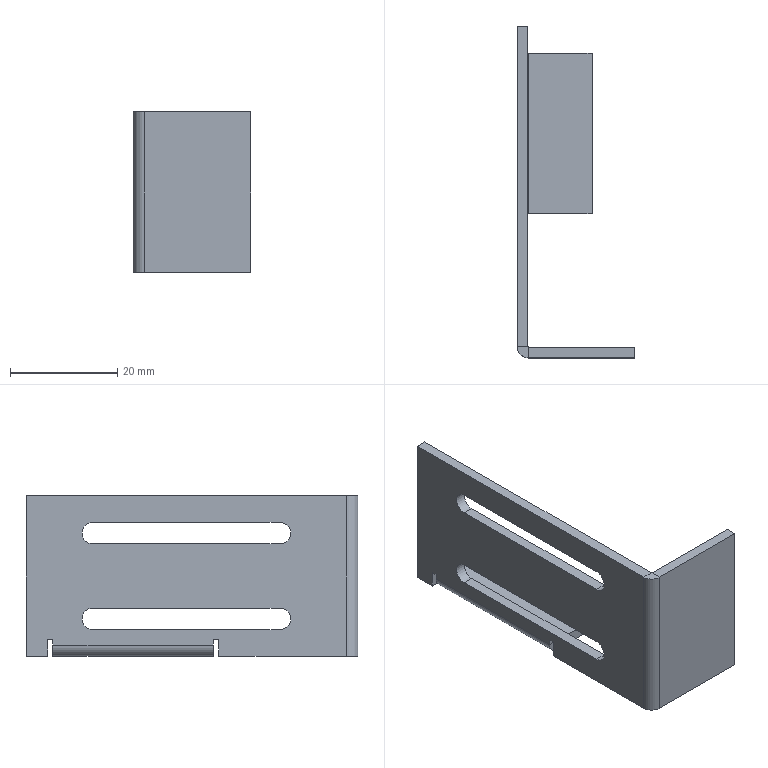Part | SolidWorks | features EdgeFlange 1, FlatPattern 1, ICE 1, SMBaseFlange 1, SheetMetal 1 | 1 solid | 40 faces | box 22 x 62 x 30 mm | volume 4961 mm3 | plane 30 | cylinder 10 | commonest cylinder face diameters 4 x6 0.2 x2 4.2 x2
STEP:
#1=CARTESIAN_POINT('',(0.,12.55,9.));
#2=VERTEX_POINT('',#1);
#3=CARTESIAN_POINT('',(0.,10.55,7.));
#4=VERTEX_POINT('',#3);
#5=CARTESIAN_POINT('',(0.,12.55,7.));
#6=DIRECTION('',(1.,0.,0.));
#7=DIRECTION('',(0.,1.,0.));
#8=AXIS2_PLACEMENT_3D('',#5,#6,#7);
#9=CIRCLE('',#8,2.);
#10=EDGE_CURVE('',#2,#4,#9,.T.);
#11=ORIENTED_EDGE('',*,*,#10,.T.);
#12=CARTESIAN_POINT('',(-2.,10.55,7.));
#13=VERTEX_POINT('',#12);
#14=CARTESIAN_POINT('',(20.,10.55,7.));
#15=DIRECTION('',(-1.,0.,0.));
#16=VECTOR('',#15,1000.);
#17=LINE('',#14,#16);
#18=EDGE_CURVE('',#4,#13,#17,.T.);
#19=ORIENTED_EDGE('',*,*,#18,.T.);
#20=CARTESIAN_POINT('',(-2.,12.55,9.));
#21=VERTEX_POINT('',#20);
#22=CARTESIAN_POINT('',(-2.,12.55,7.));
#23=DIRECTION('',(-1.,0.,0.));
#24=DIRECTION('',(0.,-1.,0.));
#25=AXIS2_PLACEMENT_3D('',#22,#23,#24);
#26=CIRCLE('',#25,2.);
#27=EDGE_CURVE('',#13,#21,#26,.T.);
#28=ORIENTED_EDGE('',*,*,#27,.T.);
#29=CARTESIAN_POINT('',(20.,12.55,9.));
#30=DIRECTION('',(-1.,0.,0.));
#31=VECTOR('',#30,1000.);
#32=LINE('',#29,#31);
#33=EDGE_CURVE('',#2,#21,#32,.T.);
#34=ORIENTED_EDGE('',*,*,#33,.F.);
#35=EDGE_LOOP('',(#11,#19,#28,#34));
#36=FACE_OUTER_BOUND('',#35,.T.);
#37=CARTESIAN_POINT('',(20.,12.55,7.));
#38=DIRECTION('',(-1.,0.,0.));
#39=DIRECTION('',(0.,-1.,0.));
#40=AXIS2_PLACEMENT_3D('',#37,#38,#39);
#41=CYLINDRICAL_SURFACE('',#40,2.);
#42=ADVANCED_FACE('',(#36),#41,.F.);
#43=CARTESIAN_POINT('',(0.,12.55,25.));
#44=VERTEX_POINT('',#43);
#45=CARTESIAN_POINT('',(0.,10.55,23.));
#46=VERTEX_POINT('',#45);
#47=CARTESIAN_POINT('',(0.,12.55,23.));
#48=DIRECTION('',(1.,0.,0.));
#49=DIRECTION('',(0.,1.,0.));
#50=AXIS2_PLACEMENT_3D('',#47,#48,#49);
#51=CIRCLE('',#50,2.);
#52=EDGE_CURVE('',#44,#46,#51,.T.);
#53=ORIENTED_EDGE('',*,*,#52,.T.);
#54=CARTESIAN_POINT('',(-2.,10.55,23.));
#55=VERTEX_POINT('',#54);
#56=CARTESIAN_POINT('',(20.,10.55,23.));
#57=DIRECTION('',(-1.,0.,0.));
#58=VECTOR('',#57,1000.);
#59=LINE('',#56,#58);
#60=EDGE_CURVE('',#46,#55,#59,.T.);
#61=ORIENTED_EDGE('',*,*,#60,.T.);
#62=CARTESIAN_POINT('',(-2.,12.55,25.));
#63=VERTEX_POINT('',#62);
#64=CARTESIAN_POINT('',(-2.,12.55,23.));
#65=DIRECTION('',(-1.,0.,0.));
#66=DIRECTION('',(0.,1.,0.));
#67=AXIS2_PLACEMENT_3D('',#64,#65,#66);
#68=CIRCLE('',#67,2.);
#69=EDGE_CURVE('',#55,#63,#68,.T.);
#70=ORIENTED_EDGE('',*,*,#69,.T.);
#71=CARTESIAN_POINT('',(20.,12.55,25.));
#72=DIRECTION('',(-1.,0.,0.));
#73=VECTOR('',#72,1000.);
#74=LINE('',#71,#73);
#75=EDGE_CURVE('',#44,#63,#74,.T.);
#76=ORIENTED_EDGE('',*,*,#75,.F.);
#77=EDGE_LOOP('',(#53,#61,#70,#76));
#78=FACE_OUTER_BOUND('',#77,.T.);
#79=CARTESIAN_POINT('',(20.,12.55,23.));
#80=DIRECTION('',(-1.,0.,0.));
#81=DIRECTION('',(0.,-1.,0.));
#82=AXIS2_PLACEMENT_3D('',#79,#80,#81);
#83=CYLINDRICAL_SURFACE('',#82,2.);
#84=ADVANCED_FACE('',(#78),#83,.F.);
#85=CARTESIAN_POINT('',(0.,60.,0.));
#86=VERTEX_POINT('',#85);
#87=CARTESIAN_POINT('',(0.,56.,0.));
#88=VERTEX_POINT('',#87);
#89=CARTESIAN_POINT('',(0.,60.,0.));
#90=DIRECTION('',(0.,-1.,0.));
#91=VECTOR('',#90,1000.);
#92=LINE('',#89,#91);
#93=EDGE_CURVE('',#86,#88,#92,.T.);
#94=ORIENTED_EDGE('',*,*,#93,.T.);
#95=CARTESIAN_POINT('',(-2.,56.,0.));
#96=VERTEX_POINT('',#95);
#97=CARTESIAN_POINT('',(0.,56.,0.));
#98=DIRECTION('',(-1.,0.,0.));
#99=VECTOR('',#98,1000.);
#100=LINE('',#97,#99);
#101=EDGE_CURVE('',#88,#96,#100,.T.);
#102=ORIENTED_EDGE('',*,*,#101,.T.);
#103=CARTESIAN_POINT('',(-2.,60.,0.));
#104=VERTEX_POINT('',#103);
#105=CARTESIAN_POINT('',(-2.,60.,0.));
#106=DIRECTION('',(0.,-1.,0.));
#107=VECTOR('',#106,1000.);
#108=LINE('',#105,#107);
#109=EDGE_CURVE('',#104,#96,#108,.T.);
#110=ORIENTED_EDGE('',*,*,#109,.F.);
#111=CARTESIAN_POINT('',(-2.,60.,0.));
#112=DIRECTION('',(1.,0.,0.));
#113=VECTOR('',#112,1000.);
#114=LINE('',#111,#113);
#115=EDGE_CURVE('',#104,#86,#114,.T.);
#116=ORIENTED_EDGE('',*,*,#115,.T.);
#117=EDGE_LOOP('',(#94,#102,#110,#116));
#118=FACE_OUTER_BOUND('',#117,.T.);
#119=CARTESIAN_POINT('',(0.1,-2.,0.));
#120=DIRECTION('',(0.,0.,-1.));
#121=DIRECTION('',(-1.,0.,0.));
#122=AXIS2_PLACEMENT_3D('',#119,#120,#121);
#123=PLANE('',#122);
#124=ADVANCED_FACE('',(#118),#123,.T.);
#125=CARTESIAN_POINT('',(-2.,24.,0.));
#126=VERTEX_POINT('',#125);
#127=CARTESIAN_POINT('',(-2.,0.1,0.));
#128=VERTEX_POINT('',#127);
#129=CARTESIAN_POINT('',(-2.,60.,0.));
#130=DIRECTION('',(0.,-1.,0.));
#131=VECTOR('',#130,1000.);
#132=LINE('',#129,#131);
#133=EDGE_CURVE('',#126,#128,#132,.T.);
#134=ORIENTED_EDGE('',*,*,#133,.F.);
#135=CARTESIAN_POINT('',(0.,24.,0.));
#136=VERTEX_POINT('',#135);
#137=CARTESIAN_POINT('',(0.,24.,0.));
#138=DIRECTION('',(-1.,0.,0.));
#139=VECTOR('',#138,1000.);
#140=LINE('',#137,#139);
#141=EDGE_CURVE('',#136,#126,#140,.T.);
#142=ORIENTED_EDGE('',*,*,#141,.F.);
#143=CARTESIAN_POINT('',(0.,0.1,0.));
#144=VERTEX_POINT('',#143);
#145=CARTESIAN_POINT('',(0.,60.,0.));
#146=DIRECTION('',(0.,-1.,0.));
#147=VECTOR('',#146,1000.);
#148=LINE('',#145,#147);
#149=EDGE_CURVE('',#136,#144,#148,.T.);
#150=ORIENTED_EDGE('',*,*,#149,.T.);
#151=CARTESIAN_POINT('',(0.,0.1,0.));
#152=DIRECTION('',(-1.,0.,0.));
#153=VECTOR('',#152,1000.);
#154=LINE('',#151,#153);
#155=EDGE_CURVE('',#144,#128,#154,.T.);
#156=ORIENTED_EDGE('',*,*,#155,.T.);
#157=EDGE_LOOP('',(#134,#142,#150,#156));
#158=FACE_OUTER_BOUND('',#157,.T.);
#159=CARTESIAN_POINT('',(0.1,-2.,0.));
#160=DIRECTION('',(0.,0.,-1.));
#161=DIRECTION('',(-1.,0.,0.));
#162=AXIS2_PLACEMENT_3D('',#159,#160,#161);
#163=PLANE('',#162);
#164=ADVANCED_FACE('',(#158),#163,.T.);
#165=CARTESIAN_POINT('',(0.,47.55,5.));
#166=VERTEX_POINT('',#165);
#167=CARTESIAN_POINT('',(0.,47.55,9.));
#168=VERTEX_POINT('',#167);
#169=CARTESIAN_POINT('',(0.,47.55,7.));
#170=DIRECTION('',(1.,0.,0.));
#171=DIRECTION('',(0.,1.,0.));
#172=AXIS2_PLACEMENT_3D('',#169,#170,#171);
#173=CIRCLE('',#172,2.);
#174=EDGE_CURVE('',#166,#168,#173,.T.);
#175=ORIENTED_EDGE('',*,*,#174,.F.);
#176=CARTESIAN_POINT('',(0.,12.55,5.));
#177=VERTEX_POINT('',#176);
#178=CARTESIAN_POINT('',(0.,60.,5.));
#179=DIRECTION('',(0.,1.,0.));
#180=VECTOR('',#179,1000.);
#181=LINE('',#178,#180);
#182=EDGE_CURVE('',#177,#166,#181,.T.);
#183=ORIENTED_EDGE('',*,*,#182,.F.);
#184=CARTESIAN_POINT('',(0.,12.55,7.));
#185=DIRECTION('',(1.,0.,0.));
#186=DIRECTION('',(0.,1.,0.));
#187=AXIS2_PLACEMENT_3D('',#184,#185,#186);
#188=CIRCLE('',#187,2.);
#189=EDGE_CURVE('',#4,#177,#188,.T.);
#190=ORIENTED_EDGE('',*,*,#189,.F.);
#191=ORIENTED_EDGE('',*,*,#10,.F.);
#192=CARTESIAN_POINT('',(0.,60.,9.));
#193=DIRECTION('',(0.,-1.,0.));
#194=VECTOR('',#193,1000.);
#195=LINE('',#192,#194);
#196=EDGE_CURVE('',#168,#2,#195,.T.);
#197=ORIENTED_EDGE('',*,*,#196,.F.);
#198=EDGE_LOOP('',(#175,#183,#190,#191,#197));
#199=FACE_BOUND('',#198,.T.);
#200=CARTESIAN_POINT('',(0.,47.55,21.));
#201=VERTEX_POINT('',#200);
#202=CARTESIAN_POINT('',(0.,47.55,25.));
#203=VERTEX_POINT('',#202);
#204=CARTESIAN_POINT('',(0.,47.55,23.));
#205=DIRECTION('',(1.,0.,0.));
#206=DIRECTION('',(0.,1.,0.));
#207=AXIS2_PLACEMENT_3D('',#204,#205,#206);
#208=CIRCLE('',#207,2.);
#209=EDGE_CURVE('',#201,#203,#208,.T.);
#210=ORIENTED_EDGE('',*,*,#209,.F.);
#211=CARTESIAN_POINT('',(0.,12.55,21.));
#212=VERTEX_POINT('',#211);
#213=CARTESIAN_POINT('',(0.,60.,21.));
#214=DIRECTION('',(0.,1.,0.));
#215=VECTOR('',#214,1000.);
#216=LINE('',#213,#215);
#217=EDGE_CURVE('',#212,#201,#216,.T.);
#218=ORIENTED_EDGE('',*,*,#217,.F.);
#219=CARTESIAN_POINT('',(0.,12.55,23.));
#220=DIRECTION('',(1.,0.,0.));
#221=DIRECTION('',(0.,1.,0.));
#222=AXIS2_PLACEMENT_3D('',#219,#220,#221);
#223=CIRCLE('',#222,2.);
#224=EDGE_CURVE('',#46,#212,#223,.T.);
#225=ORIENTED_EDGE('',*,*,#224,.F.);
#226=ORIENTED_EDGE('',*,*,#52,.F.);
#227=CARTESIAN_POINT('',(0.,60.,25.));
#228=DIRECTION('',(0.,-1.,0.));
#229=VECTOR('',#228,1000.);
#230=LINE('',#227,#229);
#231=EDGE_CURVE('',#203,#44,#230,.T.);
#232=ORIENTED_EDGE('',*,*,#231,.F.);
#233=EDGE_LOOP('',(#210,#218,#225,#226,#232));
#234=FACE_BOUND('',#233,.T.);
#235=CARTESIAN_POINT('',(0.,56.,3.1));
#236=VERTEX_POINT('',#235);
#237=CARTESIAN_POINT('',(0.,55.,3.1));
#238=VERTEX_POINT('',#237);
#239=CARTESIAN_POINT('',(0.,56.,3.1));
#240=DIRECTION('',(0.,-1.,0.));
#241=VECTOR('',#240,1000.);
#242=LINE('',#239,#241);
#243=EDGE_CURVE('',#236,#238,#242,.T.);
#244=ORIENTED_EDGE('',*,*,#243,.F.);
#245=CARTESIAN_POINT('',(0.,56.,0.));
#246=DIRECTION('',(0.,0.,1.));
#247=VECTOR('',#246,1000.);
#248=LINE('',#245,#247);
#249=EDGE_CURVE('',#88,#236,#248,.T.);
#250=ORIENTED_EDGE('',*,*,#249,.F.);
#251=ORIENTED_EDGE('',*,*,#93,.F.);
#252=CARTESIAN_POINT('',(0.,60.,30.));
#253=VERTEX_POINT('',#252);
#254=CARTESIAN_POINT('',(0.,60.,30.));
#255=DIRECTION('',(0.,0.,-1.));
#256=VECTOR('',#255,1000.);
#257=LINE('',#254,#256);
#258=EDGE_CURVE('',#253,#86,#257,.T.);
#259=ORIENTED_EDGE('',*,*,#258,.F.);
#260=CARTESIAN_POINT('',(0.,0.1,30.));
#261=VERTEX_POINT('',#260);
#262=CARTESIAN_POINT('',(0.,60.,30.));
#263=DIRECTION('',(0.,-1.,0.));
#264=VECTOR('',#263,1000.);
#265=LINE('',#262,#264);
#266=EDGE_CURVE('',#253,#261,#265,.T.);
#267=ORIENTED_EDGE('',*,*,#266,.T.);
#268=CARTESIAN_POINT('',(0.,0.1,30.));
#269=DIRECTION('',(0.,0.,-1.));
#270=VECTOR('',#269,1000.);
#271=LINE('',#268,#270);
#272=EDGE_CURVE('',#261,#144,#271,.T.);
#273=ORIENTED_EDGE('',*,*,#272,.T.);
#274=ORIENTED_EDGE('',*,*,#149,.F.);
#275=CARTESIAN_POINT('',(0.,24.,3.1));
#276=VERTEX_POINT('',#275);
#277=CARTESIAN_POINT('',(0.,24.,3.1));
#278=DIRECTION('',(0.,0.,-1.));
#279=VECTOR('',#278,1000.);
#280=LINE('',#277,#279);
#281=EDGE_CURVE('',#276,#136,#280,.T.);
#282=ORIENTED_EDGE('',*,*,#281,.F.);
#283=CARTESIAN_POINT('',(0.,25.,3.1));
#284=VERTEX_POINT('',#283);
#285=CARTESIAN_POINT('',(0.,25.,3.1));
#286=DIRECTION('',(0.,-1.,0.));
#287=VECTOR('',#286,1000.);
#288=LINE('',#285,#287);
#289=EDGE_CURVE('',#284,#276,#288,.T.);
#290=ORIENTED_EDGE('',*,*,#289,.F.);
#291=CARTESIAN_POINT('',(0.,25.,2.1));
#292=VERTEX_POINT('',#291);
#293=CARTESIAN_POINT('',(0.,25.,2.1));
#294=DIRECTION('',(0.,0.,1.));
#295=VECTOR('',#294,1000.);
#296=LINE('',#293,#295);
#297=EDGE_CURVE('',#292,#284,#296,.T.);
#298=ORIENTED_EDGE('',*,*,#297,.F.);
#299=CARTESIAN_POINT('',(0.,55.,2.1));
#300=VERTEX_POINT('',#299);
#301=CARTESIAN_POINT('',(0.,55.,2.1));
#302=DIRECTION('',(0.,-1.,0.));
#303=VECTOR('',#302,1000.);
#304=LINE('',#301,#303);
#305=EDGE_CURVE('',#300,#292,#304,.T.);
#306=ORIENTED_EDGE('',*,*,#305,.F.);
#307=CARTESIAN_POINT('',(0.,55.,3.1));
#308=DIRECTION('',(0.,0.,-1.));
#309=VECTOR('',#308,1000.);
#310=LINE('',#307,#309);
#311=EDGE_CURVE('',#238,#300,#310,.T.);
#312=ORIENTED_EDGE('',*,*,#311,.F.);
#313=EDGE_LOOP('',(#244,#250,#251,#259,#267,#273,#274,#282,#290,#298,#306,#312));
#314=FACE_OUTER_BOUND('',#313,.T.);
#315=CARTESIAN_POINT('',(0.,60.,30.));
#316=DIRECTION('',(1.,0.,0.));
#317=DIRECTION('',(0.,1.,0.));
#318=AXIS2_PLACEMENT_3D('',#315,#316,#317);
#319=PLANE('',#318);
#320=ADVANCED_FACE('',(#199,#234,#314),#319,.T.);
#321=CARTESIAN_POINT('',(-2.,47.55,21.));
#322=VERTEX_POINT('',#321);
#323=CARTESIAN_POINT('',(-2.,12.55,21.));
#324=VERTEX_POINT('',#323);
#325=CARTESIAN_POINT('',(-2.,47.55,21.));
#326=DIRECTION('',(0.,-1.,0.));
#327=VECTOR('',#326,1000.);
#328=LINE('',#325,#327);
#329=EDGE_CURVE('',#322,#324,#328,.T.);
#330=ORIENTED_EDGE('',*,*,#329,.F.);
#331=CARTESIAN_POINT('',(-2.,47.55,25.));
#332=VERTEX_POINT('',#331);
#333=CARTESIAN_POINT('',(-2.,47.55,23.));
#334=DIRECTION('',(-1.,0.,0.));
#335=DIRECTION('',(0.,1.,0.));
#336=AXIS2_PLACEMENT_3D('',#333,#334,#335);
#337=CIRCLE('',#336,2.);
#338=EDGE_CURVE('',#332,#322,#337,.T.);
#339=ORIENTED_EDGE('',*,*,#338,.F.);
#340=CARTESIAN_POINT('',(-2.,47.55,25.));
#341=DIRECTION('',(0.,1.,0.));
#342=VECTOR('',#341,1000.);
#343=LINE('',#340,#342);
#344=EDGE_CURVE('',#63,#332,#343,.T.);
#345=ORIENTED_EDGE('',*,*,#344,.F.);
#346=ORIENTED_EDGE('',*,*,#69,.F.);
#347=CARTESIAN_POINT('',(-2.,12.55,23.));
#348=DIRECTION('',(-1.,0.,0.));
#349=DIRECTION('',(0.,1.,0.));
#350=AXIS2_PLACEMENT_3D('',#347,#348,#349);
#351=CIRCLE('',#350,2.);
#352=EDGE_CURVE('',#324,#55,#351,.T.);
#353=ORIENTED_EDGE('',*,*,#352,.F.);
#354=EDGE_LOOP('',(#330,#339,#345,#346,#353));
#355=FACE_BOUND('',#354,.T.);
#356=CARTESIAN_POINT('',(-2.,47.55,5.));
#357=VERTEX_POINT('',#356);
#358=CARTESIAN_POINT('',(-2.,12.55,5.));
#359=VERTEX_POINT('',#358);
#360=CARTESIAN_POINT('',(-2.,47.55,5.));
#361=DIRECTION('',(0.,-1.,0.));
#362=VECTOR('',#361,1000.);
#363=LINE('',#360,#362);
#364=EDGE_CURVE('',#357,#359,#363,.T.);
#365=ORIENTED_EDGE('',*,*,#364,.F.);
#366=CARTESIAN_POINT('',(-2.,47.55,9.));
#367=VERTEX_POINT('',#366);
#368=CARTESIAN_POINT('',(-2.,47.55,7.));
#369=DIRECTION('',(-1.,0.,0.));
#370=DIRECTION('',(0.,-1.,0.));
#371=AXIS2_PLACEMENT_3D('',#368,#369,#370);
#372=CIRCLE('',#371,2.);
#373=EDGE_CURVE('',#367,#357,#372,.T.);
#374=ORIENTED_EDGE('',*,*,#373,.F.);
#375=CARTESIAN_POINT('',(-2.,47.55,9.));
#376=DIRECTION('',(0.,1.,0.));
#377=VECTOR('',#376,1000.);
#378=LINE('',#375,#377);
#379=EDGE_CURVE('',#21,#367,#378,.T.);
#380=ORIENTED_EDGE('',*,*,#379,.F.);
#381=ORIENTED_EDGE('',*,*,#27,.F.);
#382=CARTESIAN_POINT('',(-2.,12.55,7.));
#383=DIRECTION('',(-1.,0.,0.));
#384=DIRECTION('',(0.,-1.,0.));
#385=AXIS2_PLACEMENT_3D('',#382,#383,#384);
#386=CIRCLE('',#385,2.);
#387=EDGE_CURVE('',#359,#13,#386,.T.);
#388=ORIENTED_EDGE('',*,*,#387,.F.);
#389=EDGE_LOOP('',(#365,#374,#380,#381,#388));
#390=FACE_BOUND('',#389,.T.);
#391=CARTESIAN_POINT('',(-2.,56.,3.1));
#392=VERTEX_POINT('',#391);
#393=CARTESIAN_POINT('',(-2.,56.,30.));
#394=DIRECTION('',(0.,0.,-1.));
#395=VECTOR('',#394,1000.);
#396=LINE('',#393,#395);
#397=EDGE_CURVE('',#392,#96,#396,.T.);
#398=ORIENTED_EDGE('',*,*,#397,.F.);
#399=CARTESIAN_POINT('',(-2.,55.,3.1));
#400=VERTEX_POINT('',#399);
#401=CARTESIAN_POINT('',(-2.,60.,3.1));
#402=DIRECTION('',(0.,1.,0.));
#403=VECTOR('',#402,1000.);
#404=LINE('',#401,#403);
#405=EDGE_CURVE('',#400,#392,#404,.T.);
#406=ORIENTED_EDGE('',*,*,#405,.F.);
#407=CARTESIAN_POINT('',(-2.,55.,2.1));
#408=VERTEX_POINT('',#407);
#409=CARTESIAN_POINT('',(-2.,55.,30.));
#410=DIRECTION('',(0.,0.,1.));
#411=VECTOR('',#410,1000.);
#412=LINE('',#409,#411);
#413=EDGE_CURVE('',#408,#400,#412,.T.);
#414=ORIENTED_EDGE('',*,*,#413,.F.);
#415=CARTESIAN_POINT('',(-2.,25.,2.1));
#416=VERTEX_POINT('',#415);
#417=CARTESIAN_POINT('',(-2.,55.,2.1));
#418=DIRECTION('',(0.,-1.,0.));
#419=VECTOR('',#418,1000.);
#420=LINE('',#417,#419);
#421=EDGE_CURVE('',#408,#416,#420,.T.);
#422=ORIENTED_EDGE('',*,*,#421,.T.);
#423=CARTESIAN_POINT('',(-2.,25.,3.1));
#424=VERTEX_POINT('',#423);
#425=CARTESIAN_POINT('',(-2.,25.,30.));
#426=DIRECTION('',(0.,0.,-1.));
#427=VECTOR('',#426,1000.);
#428=LINE('',#425,#427);
#429=EDGE_CURVE('',#424,#416,#428,.T.);
#430=ORIENTED_EDGE('',*,*,#429,.F.);
#431=CARTESIAN_POINT('',(-2.,24.,3.1));
#432=VERTEX_POINT('',#431);
#433=CARTESIAN_POINT('',(-2.,60.,3.1));
#434=DIRECTION('',(0.,1.,0.));
#435=VECTOR('',#434,1000.);
#436=LINE('',#433,#435);
#437=EDGE_CURVE('',#432,#424,#436,.T.);
#438=ORIENTED_EDGE('',*,*,#437,.F.);
#439=CARTESIAN_POINT('',(-2.,24.,30.));
#440=DIRECTION('',(0.,0.,1.));
#441=VECTOR('',#440,1000.);
#442=LINE('',#439,#441);
#443=EDGE_CURVE('',#126,#432,#442,.T.);
#444=ORIENTED_EDGE('',*,*,#443,.F.);
#445=ORIENTED_EDGE('',*,*,#133,.T.);
#446=CARTESIAN_POINT('',(-2.,0.1,30.));
#447=VERTEX_POINT('',#446);
#448=CARTESIAN_POINT('',(-2.,0.1,30.));
#449=DIRECTION('',(0.,0.,-1.));
#450=VECTOR('',#449,1000.);
#451=LINE('',#448,#450);
#452=EDGE_CURVE('',#447,#128,#451,.T.);
#453=ORIENTED_EDGE('',*,*,#452,.F.);
#454=CARTESIAN_POINT('',(-2.,60.,30.));
#455=VERTEX_POINT('',#454);
#456=CARTESIAN_POINT('',(-2.,60.,30.));
#457=DIRECTION('',(0.,-1.,0.));
#458=VECTOR('',#457,1000.);
#459=LINE('',#456,#458);
#460=EDGE_CURVE('',#455,#447,#459,.T.);
#461=ORIENTED_EDGE('',*,*,#460,.F.);
#462=CARTESIAN_POINT('',(-2.,60.,30.));
#463=DIRECTION('',(0.,0.,-1.));
#464=VECTOR('',#463,1000.);
#465=LINE('',#462,#464);
#466=EDGE_CURVE('',#455,#104,#465,.T.);
#467=ORIENTED_EDGE('',*,*,#466,.T.);
#468=ORIENTED_EDGE('',*,*,#109,.T.);
#469=EDGE_LOOP('',(#398,#406,#414,#422,#430,#438,#444,#445,#453,#461,#467,#468));
#470=FACE_OUTER_BOUND('',#469,.T.);
#471=CARTESIAN_POINT('',(-2.,60.,30.));
#472=DIRECTION('',(1.,0.,0.));
#473=DIRECTION('',(0.,1.,0.));
#474=AXIS2_PLACEMENT_3D('',#471,#472,#473);
#475=PLANE('',#474);
#476=ADVANCED_FACE('',(#355,#390,#470),#475,.F.);
#477=CARTESIAN_POINT('',(0.1,0.,30.));
#478=VERTEX_POINT('',#477);
#479=CARTESIAN_POINT('',(0.1,-2.,30.));
#480=VERTEX_POINT('',#479);
#481=CARTESIAN_POINT('',(0.1,0.,30.));
#482=DIRECTION('',(0.,-1.,0.));
#483=VECTOR('',#482,1000.);
#484=LINE('',#481,#483);
#485=EDGE_CURVE('',#478,#480,#484,.T.);
#486=ORIENTED_EDGE('',*,*,#485,.F.);
#487=CARTESIAN_POINT('',(0.1,0.1,30.));
#488=DIRECTION('',(0.,0.,1.));
#489=DIRECTION('',(-1.,0.,0.));
#490=AXIS2_PLACEMENT_3D('',#487,#488,#489);
#491=CIRCLE('',#490,0.1);
#492=EDGE_CURVE('',#261,#478,#491,.T.);
#493=ORIENTED_EDGE('',*,*,#492,.F.);
#494=CARTESIAN_POINT('',(-2.,0.1,30.));
#495=DIRECTION('',(1.,0.,0.));
#496=VECTOR('',#495,1000.);
#497=LINE('',#494,#496);
#498=EDGE_CURVE('',#447,#261,#497,.T.);
#499=ORIENTED_EDGE('',*,*,#498,.F.);
#500=CARTESIAN_POINT('',(0.1,0.1,30.));
#501=DIRECTION('',(0.,0.,1.));
#502=DIRECTION('',(1.,0.,0.));
#503=AXIS2_PLACEMENT_3D('',#500,#501,#502);
#504=CIRCLE('',#503,2.1);
#505=EDGE_CURVE('',#447,#480,#504,.T.);
#506=ORIENTED_EDGE('',*,*,#505,.T.);
#507=EDGE_LOOP('',(#486,#493,#499,#506));
#508=FACE_OUTER_BOUND('',#507,.T.);
#509=CARTESIAN_POINT('',(0.1,0.,30.));
#510=DIRECTION('',(0.,0.,1.));
#511=DIRECTION('',(1.,0.,0.));
#512=AXIS2_PLACEMENT_3D('',#509,#510,#511);
#513=PLANE('',#512);
#514=ADVANCED_FACE('',(#508),#513,.T.);
#515=CARTESIAN_POINT('',(20.,0.,30.));
#516=VERTEX_POINT('',#515);
#517=CARTESIAN_POINT('',(0.,0.,30.));
#518=DIRECTION('',(1.,0.,0.));
#519=VECTOR('',#518,1000.);
#520=LINE('',#517,#519);
#521=EDGE_CURVE('',#478,#516,#520,.T.);
#522=ORIENTED_EDGE('',*,*,#521,.F.);
#523=ORIENTED_EDGE('',*,*,#485,.T.);
#524=CARTESIAN_POINT('',(20.,-2.,30.));
#525=VERTEX_POINT('',#524);
#526=CARTESIAN_POINT('',(0.,-2.,30.));
#527=DIRECTION('',(1.,0.,0.));
#528=VECTOR('',#527,1000.);
#529=LINE('',#526,#528);
#530=EDGE_CURVE('',#480,#525,#529,.T.);
#531=ORIENTED_EDGE('',*,*,#530,.T.);
#532=CARTESIAN_POINT('',(20.,0.,30.));
#533=DIRECTION('',(0.,-1.,0.));
#534=VECTOR('',#533,1000.);
#535=LINE('',#532,#534);
#536=EDGE_CURVE('',#516,#525,#535,.T.);
#537=ORIENTED_EDGE('',*,*,#536,.F.);
#538=EDGE_LOOP('',(#522,#523,#531,#537));
#539=FACE_OUTER_BOUND('',#538,.T.);
#540=CARTESIAN_POINT('',(-2.,0.1,30.));
#541=DIRECTION('',(0.,0.,1.));
#542=DIRECTION('',(1.,0.,0.));
#543=AXIS2_PLACEMENT_3D('',#540,#541,#542);
#544=PLANE('',#543);
#545=ADVANCED_FACE('',(#539),#544,.T.);
#546=ORIENTED_EDGE('',*,*,#155,.F.);
#547=CARTESIAN_POINT('',(0.1,0.,0.));
#548=VERTEX_POINT('',#547);
#549=CARTESIAN_POINT('',(0.1,0.1,0.));
#550=DIRECTION('',(0.,0.,1.));
#551=DIRECTION('',(-1.,0.,0.));
#552=AXIS2_PLACEMENT_3D('',#549,#550,#551);
#553=CIRCLE('',#552,0.1);
#554=EDGE_CURVE('',#144,#548,#553,.T.);
#555=ORIENTED_EDGE('',*,*,#554,.T.);
#556=CARTESIAN_POINT('',(0.1,-2.,0.));
#557=VERTEX_POINT('',#556);
#558=CARTESIAN_POINT('',(0.1,-2.,0.));
#559=DIRECTION('',(0.,1.,0.));
#560=VECTOR('',#559,1000.);
#561=LINE('',#558,#560);
#562=EDGE_CURVE('',#557,#548,#561,.T.);
#563=ORIENTED_EDGE('',*,*,#562,.F.);
#564=CARTESIAN_POINT('',(0.1,0.1,0.));
#565=DIRECTION('',(0.,0.,1.));
#566=DIRECTION('',(1.,0.,0.));
#567=AXIS2_PLACEMENT_3D('',#564,#565,#566);
#568=CIRCLE('',#567,2.1);
#569=EDGE_CURVE('',#128,#557,#568,.T.);
#570=ORIENTED_EDGE('',*,*,#569,.F.);
#571=EDGE_LOOP('',(#546,#555,#563,#570));
#572=FACE_OUTER_BOUND('',#571,.T.);
#573=CARTESIAN_POINT('',(0.,0.1,0.));
#574=DIRECTION('',(0.,0.,-1.));
#575=DIRECTION('',(-1.,0.,0.));
#576=AXIS2_PLACEMENT_3D('',#573,#574,#575);
#577=PLANE('',#576);
#578=ADVANCED_FACE('',(#572),#577,.T.);
#579=CARTESIAN_POINT('',(20.,-2.,0.));
#580=VERTEX_POINT('',#579);
#581=CARTESIAN_POINT('',(0.,-2.,0.));
#582=DIRECTION('',(1.,0.,0.));
#583=VECTOR('',#582,1000.);
#584=LINE('',#581,#583);
#585=EDGE_CURVE('',#557,#580,#584,.T.);
#586=ORIENTED_EDGE('',*,*,#585,.T.);
#587=CARTESIAN_POINT('',(20.,-2.,30.));
#588=DIRECTION('',(0.,0.,-1.));
#589=VECTOR('',#588,1000.);
#590=LINE('',#587,#589);
#591=EDGE_CURVE('',#525,#580,#590,.T.);
#592=ORIENTED_EDGE('',*,*,#591,.F.);
#593=ORIENTED_EDGE('',*,*,#530,.F.);
#594=CARTESIAN_POINT('',(0.1,-2.,30.));
#595=DIRECTION('',(0.,0.,-1.));
#596=VECTOR('',#595,1000.);
#597=LINE('',#594,#596);
#598=EDGE_CURVE('',#480,#557,#597,.T.);
#599=ORIENTED_EDGE('',*,*,#598,.T.);
#600=EDGE_LOOP('',(#586,#592,#593,#599));
#601=FACE_OUTER_BOUND('',#600,.T.);
#602=CARTESIAN_POINT('',(0.,-2.,30.));
#603=DIRECTION('',(0.,1.,0.));
#604=DIRECTION('',(0.,0.,1.));
#605=AXIS2_PLACEMENT_3D('',#602,#603,#604);
#606=PLANE('',#605);
#607=ADVANCED_FACE('',(#601),#606,.F.);
#608=CARTESIAN_POINT('',(20.,0.,0.));
#609=VERTEX_POINT('',#608);
#610=CARTESIAN_POINT('',(20.,0.,0.));
#611=DIRECTION('',(0.,-1.,0.));
#612=VECTOR('',#611,1000.);
#613=LINE('',#610,#612);
#614=EDGE_CURVE('',#609,#580,#613,.T.);
#615=ORIENTED_EDGE('',*,*,#614,.F.);
#616=CARTESIAN_POINT('',(20.,0.,30.));
#617=DIRECTION('',(0.,0.,-1.));
#618=VECTOR('',#617,1000.);
#619=LINE('',#616,#618);
#620=EDGE_CURVE('',#516,#609,#619,.T.);
#621=ORIENTED_EDGE('',*,*,#620,.F.);
#622=ORIENTED_EDGE('',*,*,#536,.T.);
#623=ORIENTED_EDGE('',*,*,#591,.T.);
#624=EDGE_LOOP('',(#615,#621,#622,#623));
#625=FACE_OUTER_BOUND('',#624,.T.);
#626=CARTESIAN_POINT('',(20.,0.,30.));
#627=DIRECTION('',(1.,0.,0.));
#628=DIRECTION('',(0.,0.,-1.));
#629=AXIS2_PLACEMENT_3D('',#626,#627,#628);
#630=PLANE('',#629);
#631=ADVANCED_FACE('',(#625),#630,.T.);
#632=CARTESIAN_POINT('',(0.,0.,0.));
#633=DIRECTION('',(1.,0.,0.));
#634=VECTOR('',#633,1000.);
#635=LINE('',#632,#634);
#636=EDGE_CURVE('',#548,#609,#635,.T.);
#637=ORIENTED_EDGE('',*,*,#636,.F.);
#638=CARTESIAN_POINT('',(0.1,0.,30.));
#639=DIRECTION('',(0.,0.,-1.));
#640=VECTOR('',#639,1000.);
#641=LINE('',#638,#640);
#642=EDGE_CURVE('',#478,#548,#641,.T.);
#643=ORIENTED_EDGE('',*,*,#642,.F.);
#644=ORIENTED_EDGE('',*,*,#521,.T.);
#645=ORIENTED_EDGE('',*,*,#620,.T.);
#646=EDGE_LOOP('',(#637,#643,#644,#645));
#647=FACE_OUTER_BOUND('',#646,.T.);
#648=CARTESIAN_POINT('',(0.,0.,30.));
#649=DIRECTION('',(0.,1.,0.));
#650=DIRECTION('',(0.,0.,1.));
#651=AXIS2_PLACEMENT_3D('',#648,#649,#650);
#652=PLANE('',#651);
#653=ADVANCED_FACE('',(#647),#652,.T.);
#654=ORIENTED_EDGE('',*,*,#554,.F.);
#655=ORIENTED_EDGE('',*,*,#272,.F.);
#656=ORIENTED_EDGE('',*,*,#492,.T.);
#657=ORIENTED_EDGE('',*,*,#642,.T.);
#658=EDGE_LOOP('',(#654,#655,#656,#657));
#659=FACE_OUTER_BOUND('',#658,.T.);
#660=CARTESIAN_POINT('',(0.1,0.1,30.));
#661=DIRECTION('',(0.,0.,-1.));
#662=DIRECTION('',(-1.,0.,0.));
#663=AXIS2_PLACEMENT_3D('',#660,#661,#662);
#664=CYLINDRICAL_SURFACE('',#663,0.1);
#665=ADVANCED_FACE('',(#659),#664,.F.);
#666=ORIENTED_EDGE('',*,*,#115,.F.);
#667=ORIENTED_EDGE('',*,*,#466,.F.);
#668=CARTESIAN_POINT('',(-2.,60.,30.));
#669=DIRECTION('',(1.,0.,0.));
#670=VECTOR('',#669,1000.);
#671=LINE('',#668,#670);
#672=EDGE_CURVE('',#455,#253,#671,.T.);
#673=ORIENTED_EDGE('',*,*,#672,.T.);
#674=ORIENTED_EDGE('',*,*,#258,.T.);
#675=EDGE_LOOP('',(#666,#667,#673,#674));
#676=FACE_OUTER_BOUND('',#675,.T.);
#677=CARTESIAN_POINT('',(-2.,60.,30.));
#678=DIRECTION('',(0.,1.,0.));
#679=DIRECTION('',(0.,0.,1.));
#680=AXIS2_PLACEMENT_3D('',#677,#678,#679);
#681=PLANE('',#680);
#682=ADVANCED_FACE('',(#676),#681,.T.);
#683=ORIENTED_EDGE('',*,*,#569,.T.);
#684=ORIENTED_EDGE('',*,*,#598,.F.);
#685=ORIENTED_EDGE('',*,*,#505,.F.);
#686=ORIENTED_EDGE('',*,*,#452,.T.);
#687=EDGE_LOOP('',(#683,#684,#685,#686));
#688=FACE_OUTER_BOUND('',#687,.T.);
#689=CARTESIAN_POINT('',(0.1,0.1,30.));
#690=DIRECTION('',(0.,0.,-1.));
#691=DIRECTION('',(-1.,0.,0.));
#692=AXIS2_PLACEMENT_3D('',#689,#690,#691);
#693=CYLINDRICAL_SURFACE('',#692,2.1);
#694=ADVANCED_FACE('',(#688),#693,.T.);
#695=ORIENTED_EDGE('',*,*,#460,.T.);
#696=ORIENTED_EDGE('',*,*,#498,.T.);
#697=ORIENTED_EDGE('',*,*,#266,.F.);
#698=ORIENTED_EDGE('',*,*,#672,.F.);
#699=EDGE_LOOP('',(#695,#696,#697,#698));
#700=FACE_OUTER_BOUND('',#699,.T.);
#701=CARTESIAN_POINT('',(0.1,0.1,30.));
#702=DIRECTION('',(0.,0.,-1.));
#703=DIRECTION('',(-1.,0.,0.));
#704=AXIS2_PLACEMENT_3D('',#701,#702,#703);
#705=PLANE('',#704);
#706=ADVANCED_FACE('',(#700),#705,.F.);
#707=ORIENTED_EDGE('',*,*,#585,.F.);
#708=ORIENTED_EDGE('',*,*,#562,.T.);
#709=ORIENTED_EDGE('',*,*,#636,.T.);
#710=ORIENTED_EDGE('',*,*,#614,.T.);
#711=EDGE_LOOP('',(#707,#708,#709,#710));
#712=FACE_OUTER_BOUND('',#711,.T.);
#713=CARTESIAN_POINT('',(0.1,0.1,0.));
#714=DIRECTION('',(0.,0.,-1.));
#715=DIRECTION('',(-1.,0.,0.));
#716=AXIS2_PLACEMENT_3D('',#713,#714,#715);
#717=PLANE('',#716);
#718=ADVANCED_FACE('',(#712),#717,.T.);
#719=ORIENTED_EDGE('',*,*,#209,.T.);
#720=CARTESIAN_POINT('',(20.,47.55,25.));
#721=DIRECTION('',(-1.,0.,0.));
#722=VECTOR('',#721,1000.);
#723=LINE('',#720,#722);
#724=EDGE_CURVE('',#203,#332,#723,.T.);
#725=ORIENTED_EDGE('',*,*,#724,.T.);
#726=ORIENTED_EDGE('',*,*,#338,.T.);
#727=CARTESIAN_POINT('',(20.,47.55,21.));
#728=DIRECTION('',(-1.,0.,0.));
#729=VECTOR('',#728,1000.);
#730=LINE('',#727,#729);
#731=EDGE_CURVE('',#201,#322,#730,.T.);
#732=ORIENTED_EDGE('',*,*,#731,.F.);
#733=EDGE_LOOP('',(#719,#725,#726,#732));
#734=FACE_OUTER_BOUND('',#733,.T.);
#735=CARTESIAN_POINT('',(20.,47.55,23.));
#736=DIRECTION('',(-1.,0.,0.));
#737=DIRECTION('',(0.,-1.,0.));
#738=AXIS2_PLACEMENT_3D('',#735,#736,#737);
#739=CYLINDRICAL_SURFACE('',#738,2.);
#740=ADVANCED_FACE('',(#734),#739,.F.);
#741=ORIENTED_EDGE('',*,*,#231,.T.);
#742=ORIENTED_EDGE('',*,*,#75,.T.);
#743=ORIENTED_EDGE('',*,*,#344,.T.);
#744=ORIENTED_EDGE('',*,*,#724,.F.);
#745=EDGE_LOOP('',(#741,#742,#743,#744));
#746=FACE_OUTER_BOUND('',#745,.T.);
#747=CARTESIAN_POINT('',(20.,47.55,25.));
#748=DIRECTION('',(0.,0.,1.));
#749=DIRECTION('',(1.,0.,0.));
#750=AXIS2_PLACEMENT_3D('',#747,#748,#749);
#751=PLANE('',#750);
#752=ADVANCED_FACE('',(#746),#751,.F.);
#753=ORIENTED_EDGE('',*,*,#60,.F.);
#754=ORIENTED_EDGE('',*,*,#224,.T.);
#755=CARTESIAN_POINT('',(20.,12.55,21.));
#756=DIRECTION('',(-1.,0.,0.));
#757=VECTOR('',#756,1000.);
#758=LINE('',#755,#757);
#759=EDGE_CURVE('',#212,#324,#758,.T.);
#760=ORIENTED_EDGE('',*,*,#759,.T.);
#761=ORIENTED_EDGE('',*,*,#352,.T.);
#762=EDGE_LOOP('',(#753,#754,#760,#761));
#763=FACE_OUTER_BOUND('',#762,.T.);
#764=CARTESIAN_POINT('',(20.,12.55,23.));
#765=DIRECTION('',(-1.,0.,0.));
#766=DIRECTION('',(0.,-1.,0.));
#767=AXIS2_PLACEMENT_3D('',#764,#765,#766);
#768=CYLINDRICAL_SURFACE('',#767,2.);
#769=ADVANCED_FACE('',(#763),#768,.F.);
#770=ORIENTED_EDGE('',*,*,#217,.T.);
#771=ORIENTED_EDGE('',*,*,#731,.T.);
#772=ORIENTED_EDGE('',*,*,#329,.T.);
#773=ORIENTED_EDGE('',*,*,#759,.F.);
#774=EDGE_LOOP('',(#770,#771,#772,#773));
#775=FACE_OUTER_BOUND('',#774,.T.);
#776=CARTESIAN_POINT('',(20.,47.55,21.));
#777=DIRECTION('',(0.,0.,-1.));
#778=DIRECTION('',(-1.,0.,0.));
#779=AXIS2_PLACEMENT_3D('',#776,#777,#778);
#780=PLANE('',#779);
#781=ADVANCED_FACE('',(#775),#780,.F.);
#782=ORIENTED_EDGE('',*,*,#174,.T.);
#783=CARTESIAN_POINT('',(20.,47.55,9.));
#784=DIRECTION('',(-1.,0.,0.));
#785=VECTOR('',#784,1000.);
#786=LINE('',#783,#785);
#787=EDGE_CURVE('',#168,#367,#786,.T.);
#788=ORIENTED_EDGE('',*,*,#787,.T.);
#789=ORIENTED_EDGE('',*,*,#373,.T.);
#790=CARTESIAN_POINT('',(20.,47.55,5.));
#791=DIRECTION('',(-1.,0.,0.));
#792=VECTOR('',#791,1000.);
#793=LINE('',#790,#792);
#794=EDGE_CURVE('',#166,#357,#793,.T.);
#795=ORIENTED_EDGE('',*,*,#794,.F.);
#796=EDGE_LOOP('',(#782,#788,#789,#795));
#797=FACE_OUTER_BOUND('',#796,.T.);
#798=CARTESIAN_POINT('',(20.,47.55,7.));
#799=DIRECTION('',(-1.,0.,0.));
#800=DIRECTION('',(0.,-1.,0.));
#801=AXIS2_PLACEMENT_3D('',#798,#799,#800);
#802=CYLINDRICAL_SURFACE('',#801,2.);
#803=ADVANCED_FACE('',(#797),#802,.F.);
#804=ORIENTED_EDGE('',*,*,#196,.T.);
#805=ORIENTED_EDGE('',*,*,#33,.T.);
#806=ORIENTED_EDGE('',*,*,#379,.T.);
#807=ORIENTED_EDGE('',*,*,#787,.F.);
#808=EDGE_LOOP('',(#804,#805,#806,#807));
#809=FACE_OUTER_BOUND('',#808,.T.);
#810=CARTESIAN_POINT('',(20.,47.55,9.));
#811=DIRECTION('',(0.,0.,1.));
#812=DIRECTION('',(1.,0.,0.));
#813=AXIS2_PLACEMENT_3D('',#810,#811,#812);
#814=PLANE('',#813);
#815=ADVANCED_FACE('',(#809),#814,.F.);
#816=ORIENTED_EDGE('',*,*,#18,.F.);
#817=ORIENTED_EDGE('',*,*,#189,.T.);
#818=CARTESIAN_POINT('',(20.,12.55,5.));
#819=DIRECTION('',(-1.,0.,0.));
#820=VECTOR('',#819,1000.);
#821=LINE('',#818,#820);
#822=EDGE_CURVE('',#177,#359,#821,.T.);
#823=ORIENTED_EDGE('',*,*,#822,.T.);
#824=ORIENTED_EDGE('',*,*,#387,.T.);
#825=EDGE_LOOP('',(#816,#817,#823,#824));
#826=FACE_OUTER_BOUND('',#825,.T.);
#827=CARTESIAN_POINT('',(20.,12.55,7.));
#828=DIRECTION('',(-1.,0.,0.));
#829=DIRECTION('',(0.,-1.,0.));
#830=AXIS2_PLACEMENT_3D('',#827,#828,#829);
#831=CYLINDRICAL_SURFACE('',#830,2.);
#832=ADVANCED_FACE('',(#826),#831,.F.);
#833=ORIENTED_EDGE('',*,*,#182,.T.);
#834=ORIENTED_EDGE('',*,*,#794,.T.);
#835=ORIENTED_EDGE('',*,*,#364,.T.);
#836=ORIENTED_EDGE('',*,*,#822,.F.);
#837=EDGE_LOOP('',(#833,#834,#835,#836));
#838=FACE_OUTER_BOUND('',#837,.T.);
#839=CARTESIAN_POINT('',(20.,47.55,5.));
#840=DIRECTION('',(0.,0.,-1.));
#841=DIRECTION('',(-1.,0.,0.));
#842=AXIS2_PLACEMENT_3D('',#839,#840,#841);
#843=PLANE('',#842);
#844=ADVANCED_FACE('',(#838),#843,.F.);
#845=CARTESIAN_POINT('',(0.,56.,3.1));
#846=DIRECTION('',(-1.,0.,0.));
#847=VECTOR('',#846,1000.);
#848=LINE('',#845,#847);
#849=EDGE_CURVE('',#236,#392,#848,.T.);
#850=ORIENTED_EDGE('',*,*,#849,.T.);
#851=ORIENTED_EDGE('',*,*,#397,.T.);
#852=ORIENTED_EDGE('',*,*,#101,.F.);
#853=ORIENTED_EDGE('',*,*,#249,.T.);
#854=EDGE_LOOP('',(#850,#851,#852,#853));
#855=FACE_OUTER_BOUND('',#854,.T.);
#856=CARTESIAN_POINT('',(0.,56.,0.));
#857=DIRECTION('',(0.,-1.,0.));
#858=DIRECTION('',(1.,0.,0.));
#859=AXIS2_PLACEMENT_3D('',#856,#857,#858);
#860=PLANE('',#859);
#861=ADVANCED_FACE('',(#855),#860,.T.);
#862=CARTESIAN_POINT('',(0.,55.,3.1));
#863=DIRECTION('',(-1.,0.,0.));
#864=VECTOR('',#863,1000.);
#865=LINE('',#862,#864);
#866=EDGE_CURVE('',#238,#400,#865,.T.);
#867=ORIENTED_EDGE('',*,*,#866,.T.);
#868=ORIENTED_EDGE('',*,*,#405,.T.);
#869=ORIENTED_EDGE('',*,*,#849,.F.);
#870=ORIENTED_EDGE('',*,*,#243,.T.);
#871=EDGE_LOOP('',(#867,#868,#869,#870));
#872=FACE_OUTER_BOUND('',#871,.T.);
#873=CARTESIAN_POINT('',(0.,56.,3.1));
#874=DIRECTION('',(0.,0.,-1.));
#875=DIRECTION('',(-1.,0.,0.));
#876=AXIS2_PLACEMENT_3D('',#873,#874,#875);
#877=PLANE('',#876);
#878=ADVANCED_FACE('',(#872),#877,.T.);
#879=CARTESIAN_POINT('',(0.,55.,2.1));
#880=DIRECTION('',(-1.,0.,0.));
#881=VECTOR('',#880,1000.);
#882=LINE('',#879,#881);
#883=EDGE_CURVE('',#300,#408,#882,.T.);
#884=ORIENTED_EDGE('',*,*,#883,.T.);
#885=ORIENTED_EDGE('',*,*,#413,.T.);
#886=ORIENTED_EDGE('',*,*,#866,.F.);
#887=ORIENTED_EDGE('',*,*,#311,.T.);
#888=EDGE_LOOP('',(#884,#885,#886,#887));
#889=FACE_OUTER_BOUND('',#888,.T.);
#890=CARTESIAN_POINT('',(0.,55.,3.1));
#891=DIRECTION('',(0.,1.,0.));
#892=DIRECTION('',(-1.,0.,0.));
#893=AXIS2_PLACEMENT_3D('',#890,#891,#892);
#894=PLANE('',#893);
#895=ADVANCED_FACE('',(#889),#894,.T.);
#896=CARTESIAN_POINT('',(0.,25.,3.1));
#897=DIRECTION('',(-1.,0.,0.));
#898=VECTOR('',#897,1000.);
#899=LINE('',#896,#898);
#900=EDGE_CURVE('',#284,#424,#899,.T.);
#901=ORIENTED_EDGE('',*,*,#900,.T.);
#902=ORIENTED_EDGE('',*,*,#429,.T.);
#903=CARTESIAN_POINT('',(0.,25.,2.1));
#904=DIRECTION('',(-1.,0.,0.));
#905=VECTOR('',#904,1000.);
#906=LINE('',#903,#905);
#907=EDGE_CURVE('',#292,#416,#906,.T.);
#908=ORIENTED_EDGE('',*,*,#907,.F.);
#909=ORIENTED_EDGE('',*,*,#297,.T.);
#910=EDGE_LOOP('',(#901,#902,#908,#909));
#911=FACE_OUTER_BOUND('',#910,.T.);
#912=CARTESIAN_POINT('',(0.,25.,2.1));
#913=DIRECTION('',(0.,-1.,0.));
#914=DIRECTION('',(1.,0.,0.));
#915=AXIS2_PLACEMENT_3D('',#912,#913,#914);
#916=PLANE('',#915);
#917=ADVANCED_FACE('',(#911),#916,.T.);
#918=CARTESIAN_POINT('',(0.,24.,3.1));
#919=DIRECTION('',(-1.,0.,0.));
#920=VECTOR('',#919,1000.);
#921=LINE('',#918,#920);
#922=EDGE_CURVE('',#276,#432,#921,.T.);
#923=ORIENTED_EDGE('',*,*,#922,.T.);
#924=ORIENTED_EDGE('',*,*,#437,.T.);
#925=ORIENTED_EDGE('',*,*,#900,.F.);
#926=ORIENTED_EDGE('',*,*,#289,.T.);
#927=EDGE_LOOP('',(#923,#924,#925,#926));
#928=FACE_OUTER_BOUND('',#927,.T.);
#929=CARTESIAN_POINT('',(0.,25.,3.1));
#930=DIRECTION('',(0.,0.,-1.));
#931=DIRECTION('',(-1.,0.,0.));
#932=AXIS2_PLACEMENT_3D('',#929,#930,#931);
#933=PLANE('',#932);
#934=ADVANCED_FACE('',(#928),#933,.T.);
#935=ORIENTED_EDGE('',*,*,#141,.T.);
#936=ORIENTED_EDGE('',*,*,#443,.T.);
#937=ORIENTED_EDGE('',*,*,#922,.F.);
#938=ORIENTED_EDGE('',*,*,#281,.T.);
#939=EDGE_LOOP('',(#935,#936,#937,#938));
#940=FACE_OUTER_BOUND('',#939,.T.);
#941=CARTESIAN_POINT('',(0.,24.,3.1));
#942=DIRECTION('',(0.,1.,0.));
#943=DIRECTION('',(-1.,0.,0.));
#944=AXIS2_PLACEMENT_3D('',#941,#942,#943);
#945=PLANE('',#944);
#946=ADVANCED_FACE('',(#940),#945,.T.);
#947=CARTESIAN_POINT('',(0.1,25.,2.));
#948=VERTEX_POINT('',#947);
#949=CARTESIAN_POINT('',(0.1,25.,0.));
#950=VERTEX_POINT('',#949);
#951=CARTESIAN_POINT('',(0.1,25.,0.));
#952=DIRECTION('',(0.,0.,-1.));
#953=VECTOR('',#952,1000.);
#954=LINE('',#951,#953);
#955=EDGE_CURVE('',#948,#950,#954,.T.);
#956=ORIENTED_EDGE('',*,*,#955,.F.);
#957=CARTESIAN_POINT('',(0.1,25.,2.1));
#958=DIRECTION('',(0.,-1.,0.));
#959=DIRECTION('',(-1.,0.,0.));
#960=AXIS2_PLACEMENT_3D('',#957,#958,#959);
#961=CIRCLE('',#960,0.1);
#962=EDGE_CURVE('',#292,#948,#961,.T.);
#963=ORIENTED_EDGE('',*,*,#962,.F.);
#964=ORIENTED_EDGE('',*,*,#907,.T.);
#965=CARTESIAN_POINT('',(0.1,25.,2.1));
#966=DIRECTION('',(0.,-1.,0.));
#967=DIRECTION('',(-1.,0.,0.));
#968=AXIS2_PLACEMENT_3D('',#965,#966,#967);
#969=CIRCLE('',#968,2.1);
#970=EDGE_CURVE('',#416,#950,#969,.T.);
#971=ORIENTED_EDGE('',*,*,#970,.T.);
#972=EDGE_LOOP('',(#956,#963,#964,#971));
#973=FACE_OUTER_BOUND('',#972,.T.);
#974=CARTESIAN_POINT('',(0.1,25.,2.1));
#975=DIRECTION('',(0.,-1.,0.));
#976=DIRECTION('',(1.,0.,0.));
#977=AXIS2_PLACEMENT_3D('',#974,#975,#976);
#978=PLANE('',#977);
#979=ADVANCED_FACE('',(#973),#978,.T.);
#980=CARTESIAN_POINT('',(0.1,55.,2.));
#981=VERTEX_POINT('',#980);
#982=CARTESIAN_POINT('',(0.1,55.,2.1));
#983=DIRECTION('',(0.,1.,0.));
#984=DIRECTION('',(-1.,0.,0.));
#985=AXIS2_PLACEMENT_3D('',#982,#983,#984);
#986=CIRCLE('',#985,0.1);
#987=EDGE_CURVE('',#981,#300,#986,.T.);
#988=ORIENTED_EDGE('',*,*,#987,.F.);
#989=CARTESIAN_POINT('',(0.1,55.,0.));
#990=VERTEX_POINT('',#989);
#991=CARTESIAN_POINT('',(0.1,55.,2.));
#992=DIRECTION('',(0.,0.,-1.));
#993=VECTOR('',#992,1000.);
#994=LINE('',#991,#993);
#995=EDGE_CURVE('',#981,#990,#994,.T.);
#996=ORIENTED_EDGE('',*,*,#995,.T.);
#997=CARTESIAN_POINT('',(0.1,55.,2.1));
#998=DIRECTION('',(0.,1.,0.));
#999=DIRECTION('',(-1.,0.,0.));
#1000=AXIS2_PLACEMENT_3D('',#997,#998,#999);
#1001=CIRCLE('',#1000,2.1);
#1002=EDGE_CURVE('',#990,#408,#1001,.T.);
#1003=ORIENTED_EDGE('',*,*,#1002,.T.);
#1004=ORIENTED_EDGE('',*,*,#883,.F.);
#1005=EDGE_LOOP('',(#988,#996,#1003,#1004));
#1006=FACE_OUTER_BOUND('',#1005,.T.);
#1007=CARTESIAN_POINT('',(0.1,55.,2.1));
#1008=DIRECTION('',(0.,-1.,0.));
#1009=DIRECTION('',(1.,0.,0.));
#1010=AXIS2_PLACEMENT_3D('',#1007,#1008,#1009);
#1011=PLANE('',#1010);
#1012=ADVANCED_FACE('',(#1006),#1011,.F.);
#1013=ORIENTED_EDGE('',*,*,#421,.F.);
#1014=ORIENTED_EDGE('',*,*,#1002,.F.);
#1015=CARTESIAN_POINT('',(0.1,25.,0.));
#1016=DIRECTION('',(0.,-1.,0.));
#1017=VECTOR('',#1016,1000.);
#1018=LINE('',#1015,#1017);
#1019=EDGE_CURVE('',#990,#950,#1018,.T.);
#1020=ORIENTED_EDGE('',*,*,#1019,.T.);
#1021=ORIENTED_EDGE('',*,*,#970,.F.);
#1022=EDGE_LOOP('',(#1013,#1014,#1020,#1021));
#1023=FACE_OUTER_BOUND('',#1022,.T.);
#1024=CARTESIAN_POINT('',(0.1,55.,2.1));
#1025=DIRECTION('',(0.,1.,0.));
#1026=DIRECTION('',(0.,0.,-1.));
#1027=AXIS2_PLACEMENT_3D('',#1024,#1025,#1026);
#1028=CYLINDRICAL_SURFACE('',#1027,2.1);
#1029=ADVANCED_FACE('',(#1023),#1028,.T.);
#1030=ORIENTED_EDGE('',*,*,#305,.T.);
#1031=ORIENTED_EDGE('',*,*,#962,.T.);
#1032=CARTESIAN_POINT('',(0.1,25.,2.));
#1033=DIRECTION('',(0.,1.,0.));
#1034=VECTOR('',#1033,1000.);
#1035=LINE('',#1032,#1034);
#1036=EDGE_CURVE('',#948,#981,#1035,.T.);
#1037=ORIENTED_EDGE('',*,*,#1036,.T.);
#1038=ORIENTED_EDGE('',*,*,#987,.T.);
#1039=EDGE_LOOP('',(#1030,#1031,#1037,#1038));
#1040=FACE_OUTER_BOUND('',#1039,.T.);
#1041=CARTESIAN_POINT('',(0.1,55.,2.1));
#1042=DIRECTION('',(0.,1.,0.));
#1043=DIRECTION('',(0.,0.,-1.));
#1044=AXIS2_PLACEMENT_3D('',#1041,#1042,#1043);
#1045=CYLINDRICAL_SURFACE('',#1044,0.1);
#1046=ADVANCED_FACE('',(#1040),#1045,.F.);
#1047=ORIENTED_EDGE('',*,*,#995,.F.);
#1048=CARTESIAN_POINT('',(12.,55.,2.));
#1049=VERTEX_POINT('',#1048);
#1050=CARTESIAN_POINT('',(12.,55.,2.));
#1051=DIRECTION('',(1.,0.,0.));
#1052=VECTOR('',#1051,1000.);
#1053=LINE('',#1050,#1052);
#1054=EDGE_CURVE('',#981,#1049,#1053,.T.);
#1055=ORIENTED_EDGE('',*,*,#1054,.T.);
#1056=CARTESIAN_POINT('',(12.,55.,0.));
#1057=VERTEX_POINT('',#1056);
#1058=CARTESIAN_POINT('',(12.,55.,0.));
#1059=DIRECTION('',(0.,0.,1.));
#1060=VECTOR('',#1059,1000.);
#1061=LINE('',#1058,#1060);
#1062=EDGE_CURVE('',#1057,#1049,#1061,.T.);
#1063=ORIENTED_EDGE('',*,*,#1062,.F.);
#1064=CARTESIAN_POINT('',(0.,55.,0.));
#1065=DIRECTION('',(1.,0.,0.));
#1066=VECTOR('',#1065,1000.);
#1067=LINE('',#1064,#1066);
#1068=EDGE_CURVE('',#990,#1057,#1067,.T.);
#1069=ORIENTED_EDGE('',*,*,#1068,.F.);
#1070=EDGE_LOOP('',(#1047,#1055,#1063,#1069));
#1071=FACE_OUTER_BOUND('',#1070,.T.);
#1072=CARTESIAN_POINT('',(12.,55.,0.));
#1073=DIRECTION('',(0.,-1.,0.));
#1074=DIRECTION('',(0.,0.,-1.));
#1075=AXIS2_PLACEMENT_3D('',#1072,#1073,#1074);
#1076=PLANE('',#1075);
#1077=ADVANCED_FACE('',(#1071),#1076,.F.);
#1078=ORIENTED_EDGE('',*,*,#955,.T.);
#1079=CARTESIAN_POINT('',(12.,25.,0.));
#1080=VERTEX_POINT('',#1079);
#1081=CARTESIAN_POINT('',(0.,25.,0.));
#1082=DIRECTION('',(-1.,0.,0.));
#1083=VECTOR('',#1082,1000.);
#1084=LINE('',#1081,#1083);
#1085=EDGE_CURVE('',#1080,#950,#1084,.T.);
#1086=ORIENTED_EDGE('',*,*,#1085,.F.);
#1087=CARTESIAN_POINT('',(12.,25.,2.));
#1088=VERTEX_POINT('',#1087);
#1089=CARTESIAN_POINT('',(12.,25.,0.));
#1090=DIRECTION('',(0.,0.,1.));
#1091=VECTOR('',#1090,1000.);
#1092=LINE('',#1089,#1091);
#1093=EDGE_CURVE('',#1080,#1088,#1092,.T.);
#1094=ORIENTED_EDGE('',*,*,#1093,.T.);
#1095=CARTESIAN_POINT('',(0.,25.,2.));
#1096=DIRECTION('',(-1.,0.,0.));
#1097=VECTOR('',#1096,1000.);
#1098=LINE('',#1095,#1097);
#1099=EDGE_CURVE('',#1088,#948,#1098,.T.);
#1100=ORIENTED_EDGE('',*,*,#1099,.T.);
#1101=EDGE_LOOP('',(#1078,#1086,#1094,#1100));
#1102=FACE_OUTER_BOUND('',#1101,.T.);
#1103=CARTESIAN_POINT('',(0.,25.,0.));
#1104=DIRECTION('',(0.,1.,0.));
#1105=DIRECTION('',(0.,0.,1.));
#1106=AXIS2_PLACEMENT_3D('',#1103,#1104,#1105);
#1107=PLANE('',#1106);
#1108=ADVANCED_FACE('',(#1102),#1107,.F.);
#1109=ORIENTED_EDGE('',*,*,#1019,.F.);
#1110=ORIENTED_EDGE('',*,*,#1068,.T.);
#1111=CARTESIAN_POINT('',(12.,0.,0.));
#1112=DIRECTION('',(0.,-1.,0.));
#1113=VECTOR('',#1112,1000.);
#1114=LINE('',#1111,#1113);
#1115=EDGE_CURVE('',#1057,#1080,#1114,.T.);
#1116=ORIENTED_EDGE('',*,*,#1115,.T.);
#1117=ORIENTED_EDGE('',*,*,#1085,.T.);
#1118=EDGE_LOOP('',(#1109,#1110,#1116,#1117));
#1119=FACE_OUTER_BOUND('',#1118,.T.);
#1120=CARTESIAN_POINT('',(0.,0.,0.));
#1121=DIRECTION('',(0.,0.,1.));
#1122=DIRECTION('',(1.,0.,0.));
#1123=AXIS2_PLACEMENT_3D('',#1120,#1121,#1122);
#1124=PLANE('',#1123);
#1125=ADVANCED_FACE('',(#1119),#1124,.F.);
#1126=ORIENTED_EDGE('',*,*,#1054,.F.);
#1127=ORIENTED_EDGE('',*,*,#1036,.F.);
#1128=ORIENTED_EDGE('',*,*,#1099,.F.);
#1129=CARTESIAN_POINT('',(12.,25.,2.));
#1130=DIRECTION('',(0.,-1.,0.));
#1131=VECTOR('',#1130,1000.);
#1132=LINE('',#1129,#1131);
#1133=EDGE_CURVE('',#1049,#1088,#1132,.T.);
#1134=ORIENTED_EDGE('',*,*,#1133,.F.);
#1135=EDGE_LOOP('',(#1126,#1127,#1128,#1134));
#1136=FACE_OUTER_BOUND('',#1135,.T.);
#1137=CARTESIAN_POINT('',(0.,0.,2.));
#1138=DIRECTION('',(0.,0.,1.));
#1139=DIRECTION('',(1.,0.,0.));
#1140=AXIS2_PLACEMENT_3D('',#1137,#1138,#1139);
#1141=PLANE('',#1140);
#1142=ADVANCED_FACE('',(#1136),#1141,.T.);
#1143=ORIENTED_EDGE('',*,*,#1133,.T.);
#1144=ORIENTED_EDGE('',*,*,#1093,.F.);
#1145=ORIENTED_EDGE('',*,*,#1115,.F.);
#1146=ORIENTED_EDGE('',*,*,#1062,.T.);
#1147=EDGE_LOOP('',(#1143,#1144,#1145,#1146));
#1148=FACE_OUTER_BOUND('',#1147,.T.);
#1149=CARTESIAN_POINT('',(12.,25.,0.));
#1150=DIRECTION('',(-1.,0.,0.));
#1151=DIRECTION('',(0.,0.,1.));
#1152=AXIS2_PLACEMENT_3D('',#1149,#1150,#1151);
#1153=PLANE('',#1152);
#1154=ADVANCED_FACE('',(#1148),#1153,.F.);
#1155=CLOSED_SHELL('',(#42,#84,#124,#164,#320,#476,#514,#545,#578,#607,#631,#653,#665,#682,#694,#706,#718,#740,#752,#769,#781,#803,#815,#832,#844,#861,#878,#895,#917,#934,#946,#979,#1012,#1029,#1046,#1077,#1108,#1125,#1142,#1154));
#1156=MANIFOLD_SOLID_BREP('',#1155);
#1157=CARTESIAN_POINT('',(0.,0.,0.));
#1158=DIRECTION('',(0.,0.,1.));
#1159=DIRECTION('',(1.,0.,0.));
#1160=AXIS2_PLACEMENT_3D('',#1157,#1158,#1159);
#1161=(LENGTH_UNIT()NAMED_UNIT(*)SI_UNIT(.MILLI.,.METRE.));
#1162=UNCERTAINTY_MEASURE_WITH_UNIT(LENGTH_MEASURE(0.00001),#1161,'','');
#1163=(NAMED_UNIT(*)PLANE_ANGLE_UNIT()SI_UNIT($,.RADIAN.));
#1164=(NAMED_UNIT(*)SI_UNIT($,.STERADIAN.)SOLID_ANGLE_UNIT());
#1165=(GEOMETRIC_REPRESENTATION_CONTEXT(3)GLOBAL_UNCERTAINTY_ASSIGNED_CONTEXT((#1162))GLOBAL_UNIT_ASSIGNED_CONTEXT((#1161,#1163,#1164))REPRESENTATION_CONTEXT('',''));
#1166=ADVANCED_BREP_SHAPE_REPRESENTATION('',(#1156,#1160),#1165);